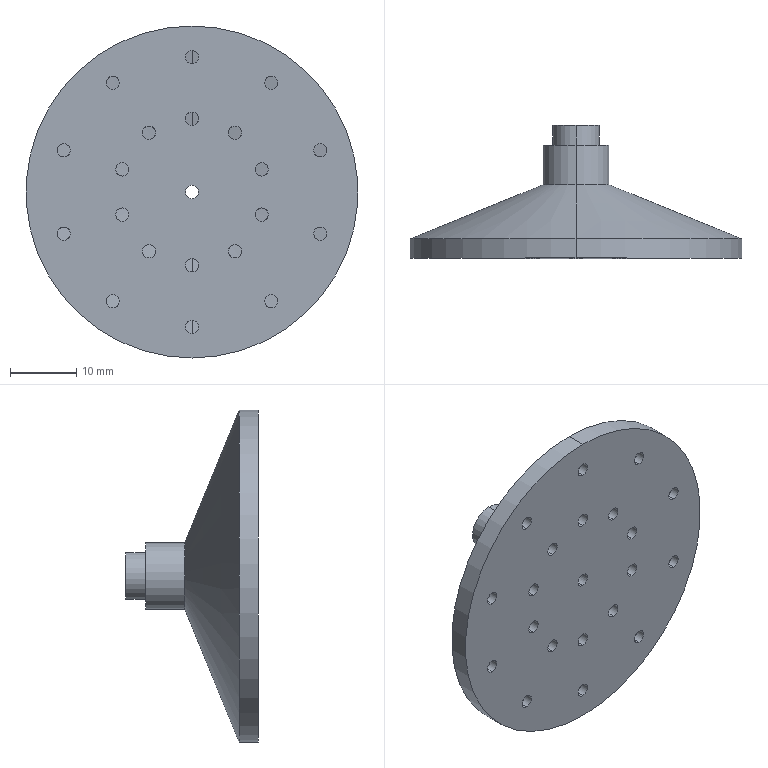Part | SolidWorks | features BaseBody 1 | 1 solid | 61 faces | box 50 x 20 x 50 mm | volume 8321 mm3 | cylinder 52 | cone 6 | plane 3 | commonest cylinder face diameters 2 x42 5 x2 7 x2 10 x2 48.449 x2 50 x2